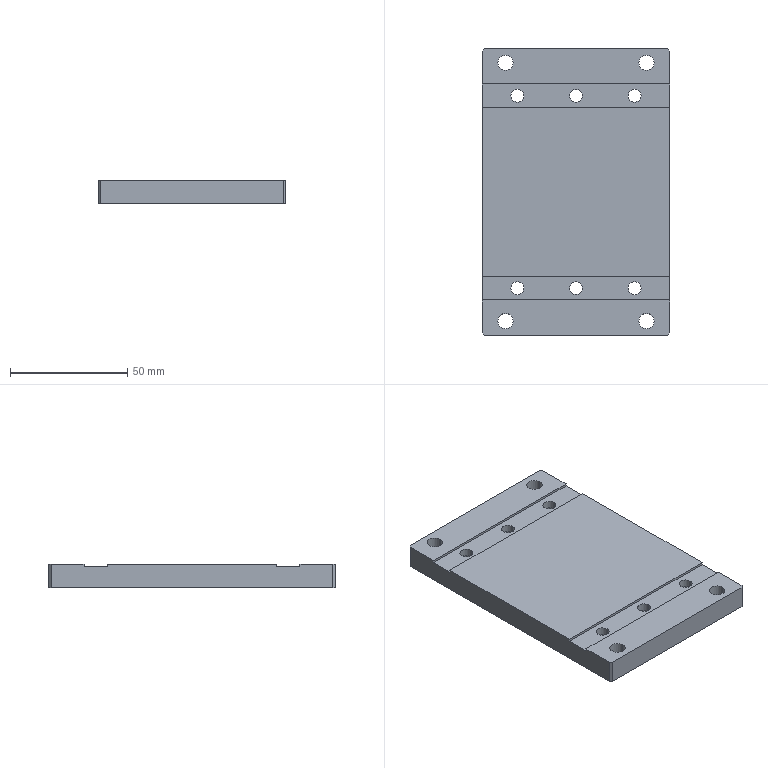Part | STEP file | 2018 Bag feed bottom plate 2 | 1 solid | 56 faces | box 80 x 122 x 10 mm | volume 91496 mm3 | cylinder 32 | plane 24 | commonest cylinder face diameters 5.5 x12 10 x12 6.5 x8